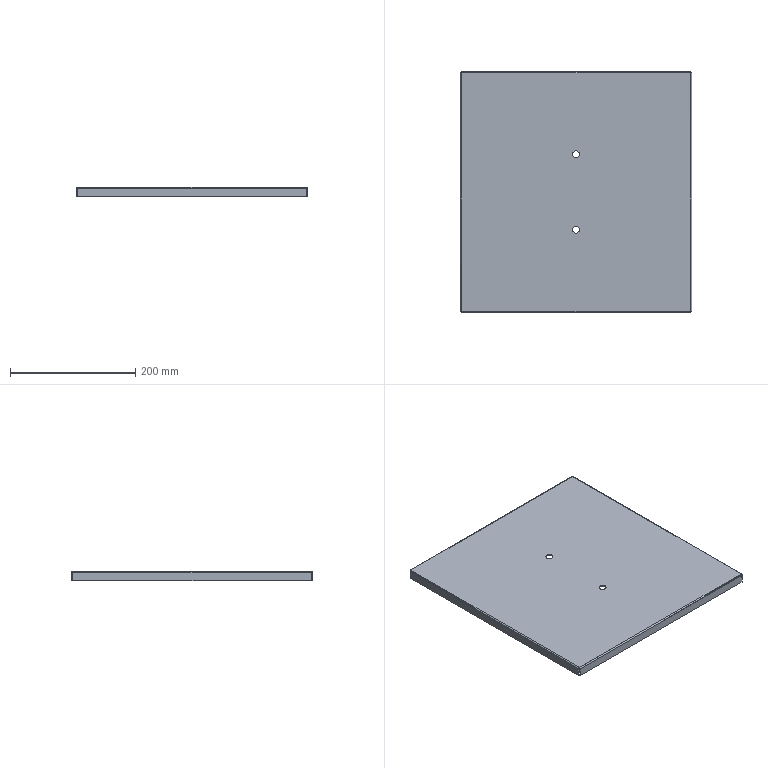Part | SolidWorks | features EdgeFlange 1, FlatPattern 1, ICE 1, SMBaseFlange 1, SheetMetal 1 | 1 solid | 42 faces | box 369 x 384 x 15 mm | volume 241174 mm3 | plane 22 | cylinder 12 | spline 8 | commonest cylinder face diameters 1 x4 4 x4 11 x4